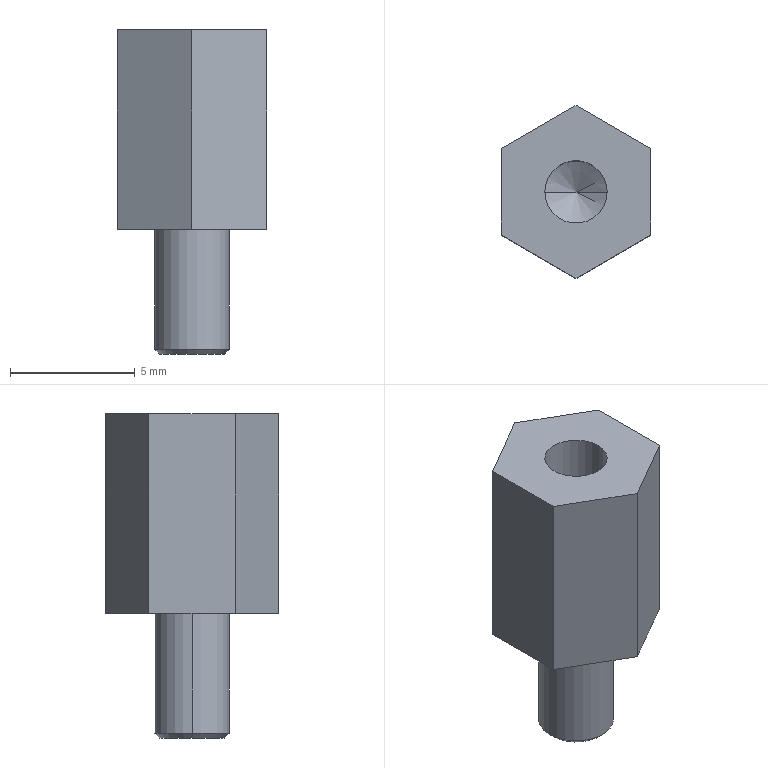Part | STEP file | Brass standoff M3-6x8 | 1 solid | 17 faces | box 6 x 6.928 x 13 mm | volume 251.442 mm3 | plane 9 | cone 4 | cylinder 4 | commonest cylinder face diameters 2.5 x2 3 x2
STEP:
#1=CARTESIAN_POINT('',(0.,0.,0.));
#2=DIRECTION('',(0.,0.,1.));
#3=DIRECTION('',(1.,0.,0.));
#4=AXIS2_PLACEMENT_3D('',#1,#2,#3);
#5=CARTESIAN_POINT('',(-1.3,0.,0.));
#6=VERTEX_POINT('',#5);
#7=CARTESIAN_POINT('',(1.3,0.,0.));
#8=VERTEX_POINT('',#7);
#9=CARTESIAN_POINT('',(0.,0.,0.));
#10=DIRECTION('',(0.,0.,-1.));
#11=DIRECTION('',(1.,0.,0.));
#12=AXIS2_PLACEMENT_3D('',#9,#10,#11);
#13=CIRCLE('',#12,1.3);
#14=CARTESIAN_POINT('',(0.,0.,0.2));
#15=DIRECTION('',(0.,0.,1.));
#16=DIRECTION('',(1.,0.,0.));
#17=AXIS2_PLACEMENT_3D('',#14,#15,#16);
#18=CONICAL_SURFACE('',#17,1.5,0.7854);
#19=CARTESIAN_POINT('',(6.283,-0.2));
#20=DIRECTION('',(-1.,0.));
#21=VECTOR('',#20,1.);
#22=LINE('',#19,#21);
#23=(GEOMETRIC_REPRESENTATION_CONTEXT(2)PARAMETRIC_REPRESENTATION_CONTEXT()REPRESENTATION_CONTEXT('',''));
#24=DEFINITIONAL_REPRESENTATION('',(#22),#23);
#25=PCURVE('',#18,#24);
#26=CARTESIAN_POINT('',(0.,0.,0.));
#27=DIRECTION('',(0.,0.,1.));
#28=DIRECTION('',(1.,0.,0.));
#29=AXIS2_PLACEMENT_3D('',#26,#27,#28);
#30=PLANE('',#29);
#31=CARTESIAN_POINT('',(1.3,0.));
#32=CARTESIAN_POINT('',(1.3,-2.252));
#33=CARTESIAN_POINT('',(-0.65,-1.126));
#34=CARTESIAN_POINT('',(-2.6,0.));
#35=CARTESIAN_POINT('',(-0.65,1.126));
#36=CARTESIAN_POINT('',(1.3,2.252));
#37=CARTESIAN_POINT('',(1.3,0.));
#38=(BOUNDED_CURVE()B_SPLINE_CURVE(2,(#31,#32,#33,#34,#35,#36,#37),.UNSPECIFIED.,.T.,.F.)B_SPLINE_CURVE_WITH_KNOTS((1,2,2,2,2,1),(-2.094,0.,2.094,4.189,6.283,8.378),.UNSPECIFIED.)CURVE()GEOMETRIC_REPRESENTATION_ITEM()RATIONAL_B_SPLINE_CURVE((1.,0.5,1.,0.5,1.,0.5,1.))REPRESENTATION_ITEM(''));
#39=(GEOMETRIC_REPRESENTATION_CONTEXT(2)PARAMETRIC_REPRESENTATION_CONTEXT()REPRESENTATION_CONTEXT('',''));
#40=DEFINITIONAL_REPRESENTATION('',(#38),#39);
#41=PCURVE('',#30,#40);
#42=SURFACE_CURVE('',#13,(#25,#41),.PCURVE_S1.);
#43=EDGE_CURVE('',#6,#8,#42,.T.);
#44=ORIENTED_EDGE('',*,*,#43,.F.);
#45=CARTESIAN_POINT('',(-1.5,0.,0.2));
#46=VERTEX_POINT('',#45);
#47=CARTESIAN_POINT('',(-1.5,0.,0.2));
#48=DIRECTION('',(-0.7071,0.,0.7071));
#49=VECTOR('',#48,1.);
#50=LINE('',#47,#49);
#51=CARTESIAN_POINT('',(3.142,0.));
#52=DIRECTION('',(0.,1.));
#53=VECTOR('',#52,1.);
#54=LINE('',#51,#53);
#55=(GEOMETRIC_REPRESENTATION_CONTEXT(2)PARAMETRIC_REPRESENTATION_CONTEXT()REPRESENTATION_CONTEXT('',''));
#56=DEFINITIONAL_REPRESENTATION('',(#54),#55);
#57=PCURVE('',#18,#56);
#58=CARTESIAN_POINT('',(0.,0.,0.2));
#59=DIRECTION('',(0.,0.,1.));
#60=DIRECTION('',(1.,0.,0.));
#61=AXIS2_PLACEMENT_3D('',#58,#59,#60);
#62=CONICAL_SURFACE('',#61,1.5,0.7854);
#63=CARTESIAN_POINT('',(3.142,0.));
#64=DIRECTION('',(0.,1.));
#65=VECTOR('',#64,1.);
#66=LINE('',#63,#65);
#67=(GEOMETRIC_REPRESENTATION_CONTEXT(2)PARAMETRIC_REPRESENTATION_CONTEXT()REPRESENTATION_CONTEXT('',''));
#68=DEFINITIONAL_REPRESENTATION('',(#66),#67);
#69=PCURVE('',#62,#68);
#70=SURFACE_CURVE('',#50,(#57,#69),.PCURVE_S1.);
#71=EDGE_CURVE('',#6,#46,#70,.T.);
#72=ORIENTED_EDGE('',*,*,#71,.T.);
#73=CARTESIAN_POINT('',(1.5,0.,0.2));
#74=VERTEX_POINT('',#73);
#75=CARTESIAN_POINT('',(0.,0.,0.2));
#76=DIRECTION('',(0.,0.,1.));
#77=DIRECTION('',(1.,0.,0.));
#78=AXIS2_PLACEMENT_3D('',#75,#76,#77);
#79=CIRCLE('',#78,1.5);
#80=CARTESIAN_POINT('',(0.,0.));
#81=DIRECTION('',(1.,0.));
#82=VECTOR('',#81,1.);
#83=LINE('',#80,#82);
#84=(GEOMETRIC_REPRESENTATION_CONTEXT(2)PARAMETRIC_REPRESENTATION_CONTEXT()REPRESENTATION_CONTEXT('',''));
#85=DEFINITIONAL_REPRESENTATION('',(#83),#84);
#86=PCURVE('',#18,#85);
#87=CARTESIAN_POINT('',(0.,0.,5.));
#88=DIRECTION('',(0.,0.,-1.));
#89=DIRECTION('',(-1.,0.,0.));
#90=AXIS2_PLACEMENT_3D('',#87,#88,#89);
#91=CYLINDRICAL_SURFACE('',#90,1.5);
#92=CARTESIAN_POINT('',(3.142,4.8));
#93=DIRECTION('',(-1.,0.));
#94=VECTOR('',#93,1.);
#95=LINE('',#92,#94);
#96=(GEOMETRIC_REPRESENTATION_CONTEXT(2)PARAMETRIC_REPRESENTATION_CONTEXT()REPRESENTATION_CONTEXT('',''));
#97=DEFINITIONAL_REPRESENTATION('',(#95),#96);
#98=PCURVE('',#91,#97);
#99=SURFACE_CURVE('',#79,(#86,#98),.PCURVE_S1.);
#100=EDGE_CURVE('',#74,#46,#99,.T.);
#101=ORIENTED_EDGE('',*,*,#100,.F.);
#102=CARTESIAN_POINT('',(1.5,0.,0.2));
#103=DIRECTION('',(0.7071,0.,0.7071));
#104=VECTOR('',#103,1.);
#105=LINE('',#102,#104);
#106=CARTESIAN_POINT('',(0.,0.));
#107=DIRECTION('',(0.,1.));
#108=VECTOR('',#107,1.);
#109=LINE('',#106,#108);
#110=(GEOMETRIC_REPRESENTATION_CONTEXT(2)PARAMETRIC_REPRESENTATION_CONTEXT()REPRESENTATION_CONTEXT('',''));
#111=DEFINITIONAL_REPRESENTATION('',(#109),#110);
#112=PCURVE('',#18,#111);
#113=CARTESIAN_POINT('',(6.283,0.));
#114=DIRECTION('',(0.,1.));
#115=VECTOR('',#114,1.);
#116=LINE('',#113,#115);
#117=(GEOMETRIC_REPRESENTATION_CONTEXT(2)PARAMETRIC_REPRESENTATION_CONTEXT()REPRESENTATION_CONTEXT('',''));
#118=DEFINITIONAL_REPRESENTATION('',(#116),#117);
#119=PCURVE('',#62,#118);
#120=SURFACE_CURVE('',#105,(#112,#119),.PCURVE_S1.);
#121=EDGE_CURVE('',#8,#74,#120,.T.);
#122=ORIENTED_EDGE('',*,*,#121,.F.);
#123=EDGE_LOOP('',(#44,#72,#101,#122));
#124=FACE_BOUND('',#123,.T.);
#125=ADVANCED_FACE('',(#124),#18,.T.);
#126=CARTESIAN_POINT('',(1.25,0.,6.5));
#127=VERTEX_POINT('',#126);
#128=CARTESIAN_POINT('',(1.25,0.,13.));
#129=VERTEX_POINT('',#128);
#130=CARTESIAN_POINT('',(1.25,0.,13.));
#131=DIRECTION('',(0.,0.,1.));
#132=VECTOR('',#131,1.);
#133=LINE('',#130,#132);
#134=CARTESIAN_POINT('',(0.,0.,13.));
#135=DIRECTION('',(0.,0.,1.));
#136=DIRECTION('',(1.,0.,0.));
#137=AXIS2_PLACEMENT_3D('',#134,#135,#136);
#138=CYLINDRICAL_SURFACE('',#137,1.25);
#139=CARTESIAN_POINT('',(6.283,0.));
#140=DIRECTION('',(0.,1.));
#141=VECTOR('',#140,1.);
#142=LINE('',#139,#141);
#143=(GEOMETRIC_REPRESENTATION_CONTEXT(2)PARAMETRIC_REPRESENTATION_CONTEXT()REPRESENTATION_CONTEXT('',''));
#144=DEFINITIONAL_REPRESENTATION('',(#142),#143);
#145=PCURVE('',#138,#144);
#146=CARTESIAN_POINT('',(0.,0.,13.));
#147=DIRECTION('',(0.,0.,1.));
#148=DIRECTION('',(1.,0.,0.));
#149=AXIS2_PLACEMENT_3D('',#146,#147,#148);
#150=CYLINDRICAL_SURFACE('',#149,1.25);
#151=CARTESIAN_POINT('',(0.,0.));
#152=DIRECTION('',(0.,1.));
#153=VECTOR('',#152,1.);
#154=LINE('',#151,#153);
#155=(GEOMETRIC_REPRESENTATION_CONTEXT(2)PARAMETRIC_REPRESENTATION_CONTEXT()REPRESENTATION_CONTEXT('',''));
#156=DEFINITIONAL_REPRESENTATION('',(#154),#155);
#157=PCURVE('',#150,#156);
#158=SURFACE_CURVE('',#133,(#145,#157),.PCURVE_S1.);
#159=EDGE_CURVE('',#127,#129,#158,.T.);
#160=ORIENTED_EDGE('',*,*,#159,.T.);
#161=CARTESIAN_POINT('',(-1.25,0.,13.));
#162=VERTEX_POINT('',#161);
#163=CARTESIAN_POINT('',(0.,0.,13.));
#164=DIRECTION('',(0.,0.,1.));
#165=DIRECTION('',(1.,0.,0.));
#166=AXIS2_PLACEMENT_3D('',#163,#164,#165);
#167=CIRCLE('',#166,1.25);
#168=CARTESIAN_POINT('',(0.,0.));
#169=DIRECTION('',(1.,0.));
#170=VECTOR('',#169,1.);
#171=LINE('',#168,#170);
#172=(GEOMETRIC_REPRESENTATION_CONTEXT(2)PARAMETRIC_REPRESENTATION_CONTEXT()REPRESENTATION_CONTEXT('',''));
#173=DEFINITIONAL_REPRESENTATION('',(#171),#172);
#174=PCURVE('',#138,#173);
#175=CARTESIAN_POINT('',(3.,-1.732,13.));
#176=DIRECTION('',(0.,0.,1.));
#177=DIRECTION('',(1.,0.,0.));
#178=AXIS2_PLACEMENT_3D('',#175,#176,#177);
#179=PLANE('',#178);
#180=CARTESIAN_POINT('',(-3.,1.732));
#181=DIRECTION('',(1.,0.));
#182=AXIS2_PLACEMENT_2D('',#180,#181);
#183=CIRCLE('',#182,1.25);
#184=(GEOMETRIC_REPRESENTATION_CONTEXT(2)PARAMETRIC_REPRESENTATION_CONTEXT()REPRESENTATION_CONTEXT('',''));
#185=DEFINITIONAL_REPRESENTATION('',(#183),#184);
#186=PCURVE('',#179,#185);
#187=SURFACE_CURVE('',#167,(#174,#186),.PCURVE_S1.);
#188=EDGE_CURVE('',#162,#129,#187,.T.);
#189=ORIENTED_EDGE('',*,*,#188,.F.);
#190=CARTESIAN_POINT('',(-1.25,0.,6.5));
#191=VERTEX_POINT('',#190);
#192=CARTESIAN_POINT('',(-1.25,0.,13.));
#193=DIRECTION('',(0.,0.,1.));
#194=VECTOR('',#193,1.);
#195=LINE('',#192,#194);
#196=CARTESIAN_POINT('',(3.142,0.));
#197=DIRECTION('',(0.,1.));
#198=VECTOR('',#197,1.);
#199=LINE('',#196,#198);
#200=(GEOMETRIC_REPRESENTATION_CONTEXT(2)PARAMETRIC_REPRESENTATION_CONTEXT()REPRESENTATION_CONTEXT('',''));
#201=DEFINITIONAL_REPRESENTATION('',(#199),#200);
#202=PCURVE('',#138,#201);
#203=CARTESIAN_POINT('',(3.142,0.));
#204=DIRECTION('',(0.,1.));
#205=VECTOR('',#204,1.);
#206=LINE('',#203,#205);
#207=(GEOMETRIC_REPRESENTATION_CONTEXT(2)PARAMETRIC_REPRESENTATION_CONTEXT()REPRESENTATION_CONTEXT('',''));
#208=DEFINITIONAL_REPRESENTATION('',(#206),#207);
#209=PCURVE('',#150,#208);
#210=SURFACE_CURVE('',#195,(#202,#209),.PCURVE_S1.);
#211=EDGE_CURVE('',#191,#162,#210,.T.);
#212=ORIENTED_EDGE('',*,*,#211,.F.);
#213=CARTESIAN_POINT('',(0.,0.,6.5));
#214=DIRECTION('',(0.,0.,1.));
#215=DIRECTION('',(1.,0.,0.));
#216=AXIS2_PLACEMENT_3D('',#213,#214,#215);
#217=CIRCLE('',#216,1.25);
#218=CARTESIAN_POINT('',(0.,-6.5));
#219=DIRECTION('',(1.,0.));
#220=VECTOR('',#219,1.);
#221=LINE('',#218,#220);
#222=(GEOMETRIC_REPRESENTATION_CONTEXT(2)PARAMETRIC_REPRESENTATION_CONTEXT()REPRESENTATION_CONTEXT('',''));
#223=DEFINITIONAL_REPRESENTATION('',(#221),#222);
#224=PCURVE('',#138,#223);
#225=CARTESIAN_POINT('',(0.,0.,6.5));
#226=DIRECTION('',(0.,0.,1.));
#227=DIRECTION('',(1.,0.,0.));
#228=AXIS2_PLACEMENT_3D('',#225,#226,#227);
#229=CONICAL_SURFACE('',#228,1.25,1.03);
#230=CARTESIAN_POINT('',(0.,0.));
#231=DIRECTION('',(1.,0.));
#232=VECTOR('',#231,1.);
#233=LINE('',#230,#232);
#234=(GEOMETRIC_REPRESENTATION_CONTEXT(2)PARAMETRIC_REPRESENTATION_CONTEXT()REPRESENTATION_CONTEXT('',''));
#235=DEFINITIONAL_REPRESENTATION('',(#233),#234);
#236=PCURVE('',#229,#235);
#237=SURFACE_CURVE('',#217,(#224,#236),.PCURVE_S1.);
#238=EDGE_CURVE('',#191,#127,#237,.T.);
#239=ORIENTED_EDGE('',*,*,#238,.T.);
#240=EDGE_LOOP('',(#160,#189,#212,#239));
#241=FACE_BOUND('',#240,.F.);
#242=ADVANCED_FACE('',(#241),#138,.F.);
#243=ORIENTED_EDGE('',*,*,#238,.F.);
#244=CARTESIAN_POINT('',(0.,0.,5.749));
#245=VERTEX_POINT('',#244);
#246=CARTESIAN_POINT('',(-1.25,0.,6.5));
#247=DIRECTION('',(-0.8572,0.,0.515));
#248=VECTOR('',#247,1.);
#249=LINE('',#246,#248);
#250=CARTESIAN_POINT('',(3.142,0.));
#251=DIRECTION('',(0.,1.));
#252=VECTOR('',#251,1.);
#253=LINE('',#250,#252);
#254=(GEOMETRIC_REPRESENTATION_CONTEXT(2)PARAMETRIC_REPRESENTATION_CONTEXT()REPRESENTATION_CONTEXT('',''));
#255=DEFINITIONAL_REPRESENTATION('',(#253),#254);
#256=PCURVE('',#229,#255);
#257=CARTESIAN_POINT('',(0.,0.,6.5));
#258=DIRECTION('',(0.,0.,1.));
#259=DIRECTION('',(1.,0.,0.));
#260=AXIS2_PLACEMENT_3D('',#257,#258,#259);
#261=CONICAL_SURFACE('',#260,1.25,1.03);
#262=CARTESIAN_POINT('',(3.142,0.));
#263=DIRECTION('',(0.,1.));
#264=VECTOR('',#263,1.);
#265=LINE('',#262,#264);
#266=(GEOMETRIC_REPRESENTATION_CONTEXT(2)PARAMETRIC_REPRESENTATION_CONTEXT()REPRESENTATION_CONTEXT('',''));
#267=DEFINITIONAL_REPRESENTATION('',(#265),#266);
#268=PCURVE('',#261,#267);
#269=SURFACE_CURVE('',#249,(#256,#268),.PCURVE_S1.);
#270=EDGE_CURVE('',#245,#191,#269,.T.);
#271=ORIENTED_EDGE('',*,*,#270,.F.);
#272=CARTESIAN_POINT('',(1.25,0.,6.5));
#273=DIRECTION('',(0.8572,0.,0.515));
#274=VECTOR('',#273,1.);
#275=LINE('',#272,#274);
#276=CARTESIAN_POINT('',(6.283,0.));
#277=DIRECTION('',(0.,1.));
#278=VECTOR('',#277,1.);
#279=LINE('',#276,#278);
#280=(GEOMETRIC_REPRESENTATION_CONTEXT(2)PARAMETRIC_REPRESENTATION_CONTEXT()REPRESENTATION_CONTEXT('',''));
#281=DEFINITIONAL_REPRESENTATION('',(#279),#280);
#282=PCURVE('',#229,#281);
#283=CARTESIAN_POINT('',(0.,0.));
#284=DIRECTION('',(0.,1.));
#285=VECTOR('',#284,1.);
#286=LINE('',#283,#285);
#287=(GEOMETRIC_REPRESENTATION_CONTEXT(2)PARAMETRIC_REPRESENTATION_CONTEXT()REPRESENTATION_CONTEXT('',''));
#288=DEFINITIONAL_REPRESENTATION('',(#286),#287);
#289=PCURVE('',#261,#288);
#290=SURFACE_CURVE('',#275,(#282,#289),.PCURVE_S1.);
#291=EDGE_CURVE('',#245,#127,#290,.T.);
#292=ORIENTED_EDGE('',*,*,#291,.T.);
#293=EDGE_LOOP('',(#243,#271,#292));
#294=FACE_BOUND('',#293,.F.);
#295=ADVANCED_FACE('',(#294),#229,.F.);
#296=CARTESIAN_POINT('',(1.5,0.,5.));
#297=VERTEX_POINT('',#296);
#298=CARTESIAN_POINT('',(-1.5,0.,5.));
#299=VERTEX_POINT('',#298);
#300=CARTESIAN_POINT('',(0.,0.,5.));
#301=DIRECTION('',(0.,0.,1.));
#302=DIRECTION('',(1.,0.,0.));
#303=AXIS2_PLACEMENT_3D('',#300,#301,#302);
#304=CIRCLE('',#303,1.5);
#305=CARTESIAN_POINT('',(3.142,0.));
#306=DIRECTION('',(-1.,0.));
#307=VECTOR('',#306,1.);
#308=LINE('',#305,#307);
#309=(GEOMETRIC_REPRESENTATION_CONTEXT(2)PARAMETRIC_REPRESENTATION_CONTEXT()REPRESENTATION_CONTEXT('',''));
#310=DEFINITIONAL_REPRESENTATION('',(#308),#309);
#311=PCURVE('',#91,#310);
#312=CARTESIAN_POINT('',(3.,-1.732,5.));
#313=DIRECTION('',(0.,0.,1.));
#314=DIRECTION('',(1.,0.,0.));
#315=AXIS2_PLACEMENT_3D('',#312,#313,#314);
#316=PLANE('',#315);
#317=CARTESIAN_POINT('',(-3.,1.732));
#318=DIRECTION('',(1.,0.));
#319=AXIS2_PLACEMENT_2D('',#317,#318);
#320=CIRCLE('',#319,1.5);
#321=(GEOMETRIC_REPRESENTATION_CONTEXT(2)PARAMETRIC_REPRESENTATION_CONTEXT()REPRESENTATION_CONTEXT('',''));
#322=DEFINITIONAL_REPRESENTATION('',(#320),#321);
#323=PCURVE('',#316,#322);
#324=SURFACE_CURVE('',#304,(#311,#323),.PCURVE_S1.);
#325=EDGE_CURVE('',#297,#299,#324,.T.);
#326=ORIENTED_EDGE('',*,*,#325,.F.);
#327=CARTESIAN_POINT('',(1.5,0.,5.));
#328=DIRECTION('',(0.,0.,-1.));
#329=VECTOR('',#328,1.);
#330=LINE('',#327,#329);
#331=CARTESIAN_POINT('',(3.142,0.));
#332=DIRECTION('',(0.,1.));
#333=VECTOR('',#332,1.);
#334=LINE('',#331,#333);
#335=(GEOMETRIC_REPRESENTATION_CONTEXT(2)PARAMETRIC_REPRESENTATION_CONTEXT()REPRESENTATION_CONTEXT('',''));
#336=DEFINITIONAL_REPRESENTATION('',(#334),#335);
#337=PCURVE('',#91,#336);
#338=CARTESIAN_POINT('',(0.,0.,5.));
#339=DIRECTION('',(0.,0.,-1.));
#340=DIRECTION('',(-1.,0.,0.));
#341=AXIS2_PLACEMENT_3D('',#338,#339,#340);
#342=CYLINDRICAL_SURFACE('',#341,1.5);
#343=CARTESIAN_POINT('',(3.142,0.));
#344=DIRECTION('',(0.,1.));
#345=VECTOR('',#344,1.);
#346=LINE('',#343,#345);
#347=(GEOMETRIC_REPRESENTATION_CONTEXT(2)PARAMETRIC_REPRESENTATION_CONTEXT()REPRESENTATION_CONTEXT('',''));
#348=DEFINITIONAL_REPRESENTATION('',(#346),#347);
#349=PCURVE('',#342,#348);
#350=SURFACE_CURVE('',#330,(#337,#349),.PCURVE_S1.);
#351=EDGE_CURVE('',#297,#74,#350,.T.);
#352=ORIENTED_EDGE('',*,*,#351,.T.);
#353=ORIENTED_EDGE('',*,*,#100,.T.);
#354=CARTESIAN_POINT('',(-1.5,0.,5.));
#355=DIRECTION('',(0.,0.,-1.));
#356=VECTOR('',#355,1.);
#357=LINE('',#354,#356);
#358=CARTESIAN_POINT('',(0.,0.));
#359=DIRECTION('',(0.,1.));
#360=VECTOR('',#359,1.);
#361=LINE('',#358,#360);
#362=(GEOMETRIC_REPRESENTATION_CONTEXT(2)PARAMETRIC_REPRESENTATION_CONTEXT()REPRESENTATION_CONTEXT('',''));
#363=DEFINITIONAL_REPRESENTATION('',(#361),#362);
#364=PCURVE('',#91,#363);
#365=CARTESIAN_POINT('',(6.283,0.));
#366=DIRECTION('',(0.,1.));
#367=VECTOR('',#366,1.);
#368=LINE('',#365,#367);
#369=(GEOMETRIC_REPRESENTATION_CONTEXT(2)PARAMETRIC_REPRESENTATION_CONTEXT()REPRESENTATION_CONTEXT('',''));
#370=DEFINITIONAL_REPRESENTATION('',(#368),#369);
#371=PCURVE('',#342,#370);
#372=SURFACE_CURVE('',#357,(#364,#371),.PCURVE_S1.);
#373=EDGE_CURVE('',#299,#46,#372,.T.);
#374=ORIENTED_EDGE('',*,*,#373,.F.);
#375=EDGE_LOOP('',(#326,#352,#353,#374));
#376=FACE_BOUND('',#375,.T.);
#377=ADVANCED_FACE('',(#376),#91,.T.);
#378=ORIENTED_EDGE('',*,*,#351,.F.);
#379=CARTESIAN_POINT('',(0.,0.,5.));
#380=DIRECTION('',(0.,0.,1.));
#381=DIRECTION('',(1.,0.,0.));
#382=AXIS2_PLACEMENT_3D('',#379,#380,#381);
#383=CIRCLE('',#382,1.5);
#384=CARTESIAN_POINT('',(9.425,0.));
#385=DIRECTION('',(-1.,0.));
#386=VECTOR('',#385,1.);
#387=LINE('',#384,#386);
#388=(GEOMETRIC_REPRESENTATION_CONTEXT(2)PARAMETRIC_REPRESENTATION_CONTEXT()REPRESENTATION_CONTEXT('',''));
#389=DEFINITIONAL_REPRESENTATION('',(#387),#388);
#390=PCURVE('',#342,#389);
#391=CARTESIAN_POINT('',(-3.,1.732));
#392=DIRECTION('',(1.,0.));
#393=AXIS2_PLACEMENT_2D('',#391,#392);
#394=CIRCLE('',#393,1.5);
#395=(GEOMETRIC_REPRESENTATION_CONTEXT(2)PARAMETRIC_REPRESENTATION_CONTEXT()REPRESENTATION_CONTEXT('',''));
#396=DEFINITIONAL_REPRESENTATION('',(#394),#395);
#397=PCURVE('',#316,#396);
#398=SURFACE_CURVE('',#383,(#390,#397),.PCURVE_S1.);
#399=EDGE_CURVE('',#299,#297,#398,.T.);
#400=ORIENTED_EDGE('',*,*,#399,.F.);
#401=ORIENTED_EDGE('',*,*,#373,.T.);
#402=CARTESIAN_POINT('',(0.,0.,0.2));
#403=DIRECTION('',(0.,0.,1.));
#404=DIRECTION('',(1.,0.,0.));
#405=AXIS2_PLACEMENT_3D('',#402,#403,#404);
#406=CIRCLE('',#405,1.5);
#407=CARTESIAN_POINT('',(9.425,4.8));
#408=DIRECTION('',(-1.,0.));
#409=VECTOR('',#408,1.);
#410=LINE('',#407,#409);
#411=(GEOMETRIC_REPRESENTATION_CONTEXT(2)PARAMETRIC_REPRESENTATION_CONTEXT()REPRESENTATION_CONTEXT('',''));
#412=DEFINITIONAL_REPRESENTATION('',(#410),#411);
#413=PCURVE('',#342,#412);
#414=CARTESIAN_POINT('',(0.,0.));
#415=DIRECTION('',(1.,0.));
#416=VECTOR('',#415,1.);
#417=LINE('',#414,#416);
#418=(GEOMETRIC_REPRESENTATION_CONTEXT(2)PARAMETRIC_REPRESENTATION_CONTEXT()REPRESENTATION_CONTEXT('',''));
#419=DEFINITIONAL_REPRESENTATION('',(#417),#418);
#420=PCURVE('',#62,#419);
#421=SURFACE_CURVE('',#406,(#413,#420),.PCURVE_S1.);
#422=EDGE_CURVE('',#46,#74,#421,.T.);
#423=ORIENTED_EDGE('',*,*,#422,.T.);
#424=EDGE_LOOP('',(#378,#400,#401,#423));
#425=FACE_BOUND('',#424,.T.);
#426=ADVANCED_FACE('',(#425),#342,.T.);
#427=CARTESIAN_POINT('',(0.,0.,0.));
#428=DIRECTION('',(0.,0.,-1.));
#429=DIRECTION('',(1.,0.,0.));
#430=AXIS2_PLACEMENT_3D('',#427,#428,#429);
#431=CIRCLE('',#430,1.3);
#432=CARTESIAN_POINT('',(1.3,0.));
#433=CARTESIAN_POINT('',(1.3,-2.252));
#434=CARTESIAN_POINT('',(-0.65,-1.126));
#435=CARTESIAN_POINT('',(-2.6,0.));
#436=CARTESIAN_POINT('',(-0.65,1.126));
#437=CARTESIAN_POINT('',(1.3,2.252));
#438=CARTESIAN_POINT('',(1.3,0.));
#439=(BOUNDED_CURVE()B_SPLINE_CURVE(2,(#432,#433,#434,#435,#436,#437,#438),.UNSPECIFIED.,.T.,.F.)B_SPLINE_CURVE_WITH_KNOTS((1,2,2,2,2,1),(-2.094,0.,2.094,4.189,6.283,8.378),.UNSPECIFIED.)CURVE()GEOMETRIC_REPRESENTATION_ITEM()RATIONAL_B_SPLINE_CURVE((1.,0.5,1.,0.5,1.,0.5,1.))REPRESENTATION_ITEM(''));
#440=(GEOMETRIC_REPRESENTATION_CONTEXT(2)PARAMETRIC_REPRESENTATION_CONTEXT()REPRESENTATION_CONTEXT('',''));
#441=DEFINITIONAL_REPRESENTATION('',(#439),#440);
#442=PCURVE('',#30,#441);
#443=CARTESIAN_POINT('',(6.283,-0.2));
#444=DIRECTION('',(-1.,0.));
#445=VECTOR('',#444,1.);
#446=LINE('',#443,#445);
#447=(GEOMETRIC_REPRESENTATION_CONTEXT(2)PARAMETRIC_REPRESENTATION_CONTEXT()REPRESENTATION_CONTEXT('',''));
#448=DEFINITIONAL_REPRESENTATION('',(#446),#447);
#449=PCURVE('',#62,#448);
#450=SURFACE_CURVE('',#431,(#442,#449),.PCURVE_S1.);
#451=EDGE_CURVE('',#8,#6,#450,.T.);
#452=ORIENTED_EDGE('',*,*,#451,.T.);
#453=ORIENTED_EDGE('',*,*,#43,.T.);
#454=EDGE_LOOP('',(#452,#453));
#455=FACE_BOUND('',#454,.T.);
#456=ADVANCED_FACE('',(#455),#30,.F.);
#457=CARTESIAN_POINT('',(0.,-3.464,5.));
#458=VERTEX_POINT('',#457);
#459=CARTESIAN_POINT('',(3.,-1.732,5.));
#460=VERTEX_POINT('',#459);
#461=CARTESIAN_POINT('',(0.,-3.464,5.));
#462=DIRECTION('',(0.866,0.5,0.));
#463=VECTOR('',#462,1.);
#464=LINE('',#461,#463);
#465=CARTESIAN_POINT('',(-3.,-1.732));
#466=DIRECTION('',(0.866,0.5));
#467=VECTOR('',#466,1.);
#468=LINE('',#465,#467);
#469=(GEOMETRIC_REPRESENTATION_CONTEXT(2)PARAMETRIC_REPRESENTATION_CONTEXT()REPRESENTATION_CONTEXT('',''));
#470=DEFINITIONAL_REPRESENTATION('',(#468),#469);
#471=PCURVE('',#316,#470);
#472=CARTESIAN_POINT('',(0.,-3.464,13.));
#473=DIRECTION('',(-0.5,0.866,0.));
#474=DIRECTION('',(-0.866,-0.5,0.));
#475=AXIS2_PLACEMENT_3D('',#472,#473,#474);
#476=PLANE('',#475);
#477=CARTESIAN_POINT('',(0.,-8.));
#478=DIRECTION('',(-1.,0.));
#479=VECTOR('',#478,1.);
#480=LINE('',#477,#479);
#481=(GEOMETRIC_REPRESENTATION_CONTEXT(2)PARAMETRIC_REPRESENTATION_CONTEXT()REPRESENTATION_CONTEXT('',''));
#482=DEFINITIONAL_REPRESENTATION('',(#480),#481);
#483=PCURVE('',#476,#482);
#484=SURFACE_CURVE('',#464,(#471,#483),.PCURVE_S1.);
#485=EDGE_CURVE('',#458,#460,#484,.T.);
#486=ORIENTED_EDGE('',*,*,#485,.F.);
#487=CARTESIAN_POINT('',(-3.,-1.732,5.));
#488=VERTEX_POINT('',#487);
#489=CARTESIAN_POINT('',(-3.,-1.732,5.));
#490=DIRECTION('',(0.866,-0.5,0.));
#491=VECTOR('',#490,1.);
#492=LINE('',#489,#491);
#493=CARTESIAN_POINT('',(-6.,0.));
#494=DIRECTION('',(0.866,-0.5));
#495=VECTOR('',#494,1.);
#496=LINE('',#493,#495);
#497=(GEOMETRIC_REPRESENTATION_CONTEXT(2)PARAMETRIC_REPRESENTATION_CONTEXT()REPRESENTATION_CONTEXT('',''));
#498=DEFINITIONAL_REPRESENTATION('',(#496),#497);
#499=PCURVE('',#316,#498);
#500=CARTESIAN_POINT('',(-3.,-1.732,13.));
#501=DIRECTION('',(0.5,0.866,0.));
#502=DIRECTION('',(-0.866,0.5,0.));
#503=AXIS2_PLACEMENT_3D('',#500,#501,#502);
#504=PLANE('',#503);
#505=CARTESIAN_POINT('',(0.,-8.));
#506=DIRECTION('',(-1.,0.));
#507=VECTOR('',#506,1.);
#508=LINE('',#505,#507);
#509=(GEOMETRIC_REPRESENTATION_CONTEXT(2)PARAMETRIC_REPRESENTATION_CONTEXT()REPRESENTATION_CONTEXT('',''));
#510=DEFINITIONAL_REPRESENTATION('',(#508),#509);
#511=PCURVE('',#504,#510);
#512=SURFACE_CURVE('',#492,(#499,#511),.PCURVE_S1.);
#513=EDGE_CURVE('',#488,#458,#512,.T.);
#514=ORIENTED_EDGE('',*,*,#513,.F.);
#515=CARTESIAN_POINT('',(-3.,1.732,5.));
#516=VERTEX_POINT('',#515);
#517=CARTESIAN_POINT('',(-3.,1.732,5.));
#518=DIRECTION('',(0.,-1.,0.));
#519=VECTOR('',#518,1.);
#520=LINE('',#517,#519);
#521=CARTESIAN_POINT('',(-6.,3.464));
#522=DIRECTION('',(0.,-1.));
#523=VECTOR('',#522,1.);
#524=LINE('',#521,#523);
#525=(GEOMETRIC_REPRESENTATION_CONTEXT(2)PARAMETRIC_REPRESENTATION_CONTEXT()REPRESENTATION_CONTEXT('',''));
#526=DEFINITIONAL_REPRESENTATION('',(#524),#525);
#527=PCURVE('',#316,#526);
#528=CARTESIAN_POINT('',(-3.,1.732,13.));
#529=DIRECTION('',(1.,0.,0.));
#530=DIRECTION('',(0.,0.,-1.));
#531=AXIS2_PLACEMENT_3D('',#528,#529,#530);
#532=PLANE('',#531);
#533=CARTESIAN_POINT('',(8.,0.));
#534=DIRECTION('',(0.,-1.));
#535=VECTOR('',#534,1.);
#536=LINE('',#533,#535);
#537=(GEOMETRIC_REPRESENTATION_CONTEXT(2)PARAMETRIC_REPRESENTATION_CONTEXT()REPRESENTATION_CONTEXT('',''));
#538=DEFINITIONAL_REPRESENTATION('',(#536),#537);
#539=PCURVE('',#532,#538);
#540=SURFACE_CURVE('',#520,(#527,#539),.PCURVE_S1.);
#541=EDGE_CURVE('',#516,#488,#540,.T.);
#542=ORIENTED_EDGE('',*,*,#541,.F.);
#543=CARTESIAN_POINT('',(0.,3.464,5.));
#544=VERTEX_POINT('',#543);
#545=CARTESIAN_POINT('',(0.,3.464,5.));
#546=DIRECTION('',(-0.866,-0.5,0.));
#547=VECTOR('',#546,1.);
#548=LINE('',#545,#547);
#549=CARTESIAN_POINT('',(-3.,5.196));
#550=DIRECTION('',(-0.866,-0.5));
#551=VECTOR('',#550,1.);
#552=LINE('',#549,#551);
#553=(GEOMETRIC_REPRESENTATION_CONTEXT(2)PARAMETRIC_REPRESENTATION_CONTEXT()REPRESENTATION_CONTEXT('',''));
#554=DEFINITIONAL_REPRESENTATION('',(#552),#553);
#555=PCURVE('',#316,#554);
#556=CARTESIAN_POINT('',(0.,3.464,13.));
#557=DIRECTION('',(0.5,-0.866,0.));
#558=DIRECTION('',(0.866,0.5,0.));
#559=AXIS2_PLACEMENT_3D('',#556,#557,#558);
#560=PLANE('',#559);
#561=CARTESIAN_POINT('',(0.,-8.));
#562=DIRECTION('',(-1.,0.));
#563=VECTOR('',#562,1.);
#564=LINE('',#561,#563);
#565=(GEOMETRIC_REPRESENTATION_CONTEXT(2)PARAMETRIC_REPRESENTATION_CONTEXT()REPRESENTATION_CONTEXT('',''));
#566=DEFINITIONAL_REPRESENTATION('',(#564),#565);
#567=PCURVE('',#560,#566);
#568=SURFACE_CURVE('',#548,(#555,#567),.PCURVE_S1.);
#569=EDGE_CURVE('',#544,#516,#568,.T.);
#570=ORIENTED_EDGE('',*,*,#569,.F.);
#571=CARTESIAN_POINT('',(3.,1.732,5.));
#572=VERTEX_POINT('',#571);
#573=CARTESIAN_POINT('',(3.,1.732,5.));
#574=DIRECTION('',(-0.866,0.5,0.));
#575=VECTOR('',#574,1.);
#576=LINE('',#573,#575);
#577=CARTESIAN_POINT('',(0.,3.464));
#578=DIRECTION('',(-0.866,0.5));
#579=VECTOR('',#578,1.);
#580=LINE('',#577,#579);
#581=(GEOMETRIC_REPRESENTATION_CONTEXT(2)PARAMETRIC_REPRESENTATION_CONTEXT()REPRESENTATION_CONTEXT('',''));
#582=DEFINITIONAL_REPRESENTATION('',(#580),#581);
#583=PCURVE('',#316,#582);
#584=CARTESIAN_POINT('',(3.,1.732,13.));
#585=DIRECTION('',(-0.5,-0.866,0.));
#586=DIRECTION('',(0.866,-0.5,0.));
#587=AXIS2_PLACEMENT_3D('',#584,#585,#586);
#588=PLANE('',#587);
#589=CARTESIAN_POINT('',(0.,-8.));
#590=DIRECTION('',(-1.,0.));
#591=VECTOR('',#590,1.);
#592=LINE('',#589,#591);
#593=(GEOMETRIC_REPRESENTATION_CONTEXT(2)PARAMETRIC_REPRESENTATION_CONTEXT()REPRESENTATION_CONTEXT('',''));
#594=DEFINITIONAL_REPRESENTATION('',(#592),#593);
#595=PCURVE('',#588,#594);
#596=SURFACE_CURVE('',#576,(#583,#595),.PCURVE_S1.);
#597=EDGE_CURVE('',#572,#544,#596,.T.);
#598=ORIENTED_EDGE('',*,*,#597,.F.);
#599=CARTESIAN_POINT('',(3.,-1.732,5.));
#600=DIRECTION('',(0.,1.,0.));
#601=VECTOR('',#600,1.);
#602=LINE('',#599,#601);
#603=CARTESIAN_POINT('',(0.,0.));
#604=DIRECTION('',(0.,1.));
#605=VECTOR('',#604,1.);
#606=LINE('',#603,#605);
#607=(GEOMETRIC_REPRESENTATION_CONTEXT(2)PARAMETRIC_REPRESENTATION_CONTEXT()REPRESENTATION_CONTEXT('',''));
#608=DEFINITIONAL_REPRESENTATION('',(#606),#607);
#609=PCURVE('',#316,#608);
#610=CARTESIAN_POINT('',(3.,-1.732,13.));
#611=DIRECTION('',(-1.,0.,0.));
#612=DIRECTION('',(0.,0.,1.));
#613=AXIS2_PLACEMENT_3D('',#610,#611,#612);
#614=PLANE('',#613);
#615=CARTESIAN_POINT('',(-8.,0.));
#616=DIRECTION('',(0.,1.));
#617=VECTOR('',#616,1.);
#618=LINE('',#615,#617);
#619=(GEOMETRIC_REPRESENTATION_CONTEXT(2)PARAMETRIC_REPRESENTATION_CONTEXT()REPRESENTATION_CONTEXT('',''));
#620=DEFINITIONAL_REPRESENTATION('',(#618),#619);
#621=PCURVE('',#614,#620);
#622=SURFACE_CURVE('',#602,(#609,#621),.PCURVE_S1.);
#623=EDGE_CURVE('',#460,#572,#622,.T.);
#624=ORIENTED_EDGE('',*,*,#623,.F.);
#625=EDGE_LOOP('',(#486,#514,#542,#570,#598,#624));
#626=FACE_BOUND('',#625,.T.);
#627=ORIENTED_EDGE('',*,*,#399,.T.);
#628=ORIENTED_EDGE('',*,*,#325,.T.);
#629=EDGE_LOOP('',(#627,#628));
#630=FACE_BOUND('',#629,.T.);
#631=ADVANCED_FACE('',(#626,#630),#316,.F.);
#632=ORIENTED_EDGE('',*,*,#485,.T.);
#633=CARTESIAN_POINT('',(3.,-1.732,13.));
#634=VERTEX_POINT('',#633);
#635=CARTESIAN_POINT('',(3.,-1.732,13.));
#636=DIRECTION('',(0.,0.,-1.));
#637=VECTOR('',#636,1.);
#638=LINE('',#635,#637);
#639=CARTESIAN_POINT('',(-3.464,0.));
#640=DIRECTION('',(0.,-1.));
#641=VECTOR('',#640,1.);
#642=LINE('',#639,#641);
#643=(GEOMETRIC_REPRESENTATION_CONTEXT(2)PARAMETRIC_REPRESENTATION_CONTEXT()REPRESENTATION_CONTEXT('',''));
#644=DEFINITIONAL_REPRESENTATION('',(#642),#643);
#645=PCURVE('',#476,#644);
#646=CARTESIAN_POINT('',(0.,0.));
#647=DIRECTION('',(-1.,0.));
#648=VECTOR('',#647,1.);
#649=LINE('',#646,#648);
#650=(GEOMETRIC_REPRESENTATION_CONTEXT(2)PARAMETRIC_REPRESENTATION_CONTEXT()REPRESENTATION_CONTEXT('',''));
#651=DEFINITIONAL_REPRESENTATION('',(#649),#650);
#652=PCURVE('',#614,#651);
#653=SURFACE_CURVE('',#638,(#645,#652),.PCURVE_S1.);
#654=EDGE_CURVE('',#634,#460,#653,.T.);
#655=ORIENTED_EDGE('',*,*,#654,.F.);
#656=CARTESIAN_POINT('',(0.,-3.464,13.));
#657=VERTEX_POINT('',#656);
#658=CARTESIAN_POINT('',(0.,-3.464,13.));
#659=DIRECTION('',(0.866,0.5,0.));
#660=VECTOR('',#659,1.);
#661=LINE('',#658,#660);
#662=CARTESIAN_POINT('',(0.,0.));
#663=DIRECTION('',(-1.,0.));
#664=VECTOR('',#663,1.);
#665=LINE('',#662,#664);
#666=(GEOMETRIC_REPRESENTATION_CONTEXT(2)PARAMETRIC_REPRESENTATION_CONTEXT()REPRESENTATION_CONTEXT('',''));
#667=DEFINITIONAL_REPRESENTATION('',(#665),#666);
#668=PCURVE('',#476,#667);
#669=CARTESIAN_POINT('',(-3.,-1.732));
#670=DIRECTION('',(0.866,0.5));
#671=VECTOR('',#670,1.);
#672=LINE('',#669,#671);
#673=(GEOMETRIC_REPRESENTATION_CONTEXT(2)PARAMETRIC_REPRESENTATION_CONTEXT()REPRESENTATION_CONTEXT('',''));
#674=DEFINITIONAL_REPRESENTATION('',(#672),#673);
#675=PCURVE('',#179,#674);
#676=SURFACE_CURVE('',#661,(#668,#675),.PCURVE_S1.);
#677=EDGE_CURVE('',#657,#634,#676,.T.);
#678=ORIENTED_EDGE('',*,*,#677,.F.);
#679=CARTESIAN_POINT('',(0.,-3.464,13.));
#680=DIRECTION('',(0.,0.,-1.));
#681=VECTOR('',#680,1.);
#682=LINE('',#679,#681);
#683=CARTESIAN_POINT('',(0.,0.));
#684=DIRECTION('',(0.,-1.));
#685=VECTOR('',#684,1.);
#686=LINE('',#683,#685);
#687=(GEOMETRIC_REPRESENTATION_CONTEXT(2)PARAMETRIC_REPRESENTATION_CONTEXT()REPRESENTATION_CONTEXT('',''));
#688=DEFINITIONAL_REPRESENTATION('',(#686),#687);
#689=PCURVE('',#476,#688);
#690=CARTESIAN_POINT('',(-3.464,0.));
#691=DIRECTION('',(0.,-1.));
#692=VECTOR('',#691,1.);
#693=LINE('',#690,#692);
#694=(GEOMETRIC_REPRESENTATION_CONTEXT(2)PARAMETRIC_REPRESENTATION_CONTEXT()REPRESENTATION_CONTEXT('',''));
#695=DEFINITIONAL_REPRESENTATION('',(#693),#694);
#696=PCURVE('',#504,#695);
#697=SURFACE_CURVE('',#682,(#689,#696),.PCURVE_S1.);
#698=EDGE_CURVE('',#657,#458,#697,.T.);
#699=ORIENTED_EDGE('',*,*,#698,.T.);
#700=EDGE_LOOP('',(#632,#655,#678,#699));
#701=FACE_BOUND('',#700,.T.);
#702=ADVANCED_FACE('',(#701),#476,.F.);
#703=ORIENTED_EDGE('',*,*,#623,.T.);
#704=CARTESIAN_POINT('',(3.,1.732,13.));
#705=VERTEX_POINT('',#704);
#706=CARTESIAN_POINT('',(3.,1.732,13.));
#707=DIRECTION('',(0.,0.,-1.));
#708=VECTOR('',#707,1.);
#709=LINE('',#706,#708);
#710=CARTESIAN_POINT('',(0.,3.464));
#711=DIRECTION('',(-1.,0.));
#712=VECTOR('',#711,1.);
#713=LINE('',#710,#712);
#714=(GEOMETRIC_REPRESENTATION_CONTEXT(2)PARAMETRIC_REPRESENTATION_CONTEXT()REPRESENTATION_CONTEXT('',''));
#715=DEFINITIONAL_REPRESENTATION('',(#713),#714);
#716=PCURVE('',#614,#715);
#717=CARTESIAN_POINT('',(0.,0.));
#718=DIRECTION('',(0.,-1.));
#719=VECTOR('',#718,1.);
#720=LINE('',#717,#719);
#721=(GEOMETRIC_REPRESENTATION_CONTEXT(2)PARAMETRIC_REPRESENTATION_CONTEXT()REPRESENTATION_CONTEXT('',''));
#722=DEFINITIONAL_REPRESENTATION('',(#720),#721);
#723=PCURVE('',#588,#722);
#724=SURFACE_CURVE('',#709,(#716,#723),.PCURVE_S1.);
#725=EDGE_CURVE('',#705,#572,#724,.T.);
#726=ORIENTED_EDGE('',*,*,#725,.F.);
#727=CARTESIAN_POINT('',(3.,-1.732,13.));
#728=DIRECTION('',(0.,1.,0.));
#729=VECTOR('',#728,1.);
#730=LINE('',#727,#729);
#731=CARTESIAN_POINT('',(0.,0.));
#732=DIRECTION('',(0.,1.));
#733=VECTOR('',#732,1.);
#734=LINE('',#731,#733);
#735=(GEOMETRIC_REPRESENTATION_CONTEXT(2)PARAMETRIC_REPRESENTATION_CONTEXT()REPRESENTATION_CONTEXT('',''));
#736=DEFINITIONAL_REPRESENTATION('',(#734),#735);
#737=PCURVE('',#614,#736);
#738=CARTESIAN_POINT('',(0.,0.));
#739=DIRECTION('',(0.,1.));
#740=VECTOR('',#739,1.);
#741=LINE('',#738,#740);
#742=(GEOMETRIC_REPRESENTATION_CONTEXT(2)PARAMETRIC_REPRESENTATION_CONTEXT()REPRESENTATION_CONTEXT('',''));
#743=DEFINITIONAL_REPRESENTATION('',(#741),#742);
#744=PCURVE('',#179,#743);
#745=SURFACE_CURVE('',#730,(#737,#744),.PCURVE_S1.);
#746=EDGE_CURVE('',#634,#705,#745,.T.);
#747=ORIENTED_EDGE('',*,*,#746,.F.);
#748=ORIENTED_EDGE('',*,*,#654,.T.);
#749=EDGE_LOOP('',(#703,#726,#747,#748));
#750=FACE_BOUND('',#749,.T.);
#751=ADVANCED_FACE('',(#750),#614,.F.);
#752=ORIENTED_EDGE('',*,*,#597,.T.);
#753=CARTESIAN_POINT('',(0.,3.464,13.));
#754=VERTEX_POINT('',#753);
#755=CARTESIAN_POINT('',(0.,3.464,13.));
#756=DIRECTION('',(0.,0.,-1.));
#757=VECTOR('',#756,1.);
#758=LINE('',#755,#757);
#759=CARTESIAN_POINT('',(-3.464,0.));
#760=DIRECTION('',(0.,-1.));
#761=VECTOR('',#760,1.);
#762=LINE('',#759,#761);
#763=(GEOMETRIC_REPRESENTATION_CONTEXT(2)PARAMETRIC_REPRESENTATION_CONTEXT()REPRESENTATION_CONTEXT('',''));
#764=DEFINITIONAL_REPRESENTATION('',(#762),#763);
#765=PCURVE('',#588,#764);
#766=CARTESIAN_POINT('',(0.,0.));
#767=DIRECTION('',(0.,-1.));
#768=VECTOR('',#767,1.);
#769=LINE('',#766,#768);
#770=(GEOMETRIC_REPRESENTATION_CONTEXT(2)PARAMETRIC_REPRESENTATION_CONTEXT()REPRESENTATION_CONTEXT('',''));
#771=DEFINITIONAL_REPRESENTATION('',(#769),#770);
#772=PCURVE('',#560,#771);
#773=SURFACE_CURVE('',#758,(#765,#772),.PCURVE_S1.);
#774=EDGE_CURVE('',#754,#544,#773,.T.);
#775=ORIENTED_EDGE('',*,*,#774,.F.);
#776=CARTESIAN_POINT('',(3.,1.732,13.));
#777=DIRECTION('',(-0.866,0.5,0.));
#778=VECTOR('',#777,1.);
#779=LINE('',#776,#778);
#780=CARTESIAN_POINT('',(0.,0.));
#781=DIRECTION('',(-1.,0.));
#782=VECTOR('',#781,1.);
#783=LINE('',#780,#782);
#784=(GEOMETRIC_REPRESENTATION_CONTEXT(2)PARAMETRIC_REPRESENTATION_CONTEXT()REPRESENTATION_CONTEXT('',''));
#785=DEFINITIONAL_REPRESENTATION('',(#783),#784);
#786=PCURVE('',#588,#785);
#787=CARTESIAN_POINT('',(0.,3.464));
#788=DIRECTION('',(-0.866,0.5));
#789=VECTOR('',#788,1.);
#790=LINE('',#787,#789);
#791=(GEOMETRIC_REPRESENTATION_CONTEXT(2)PARAMETRIC_REPRESENTATION_CONTEXT()REPRESENTATION_CONTEXT('',''));
#792=DEFINITIONAL_REPRESENTATION('',(#790),#791);
#793=PCURVE('',#179,#792);
#794=SURFACE_CURVE('',#779,(#786,#793),.PCURVE_S1.);
#795=EDGE_CURVE('',#705,#754,#794,.T.);
#796=ORIENTED_EDGE('',*,*,#795,.F.);
#797=ORIENTED_EDGE('',*,*,#725,.T.);
#798=EDGE_LOOP('',(#752,#775,#796,#797));
#799=FACE_BOUND('',#798,.T.);
#800=ADVANCED_FACE('',(#799),#588,.F.);
#801=ORIENTED_EDGE('',*,*,#569,.T.);
#802=CARTESIAN_POINT('',(-3.,1.732,13.));
#803=VERTEX_POINT('',#802);
#804=CARTESIAN_POINT('',(-3.,1.732,13.));
#805=DIRECTION('',(0.,0.,-1.));
#806=VECTOR('',#805,1.);
#807=LINE('',#804,#806);
#808=CARTESIAN_POINT('',(-3.464,0.));
#809=DIRECTION('',(0.,-1.));
#810=VECTOR('',#809,1.);
#811=LINE('',#808,#810);
#812=(GEOMETRIC_REPRESENTATION_CONTEXT(2)PARAMETRIC_REPRESENTATION_CONTEXT()REPRESENTATION_CONTEXT('',''));
#813=DEFINITIONAL_REPRESENTATION('',(#811),#812);
#814=PCURVE('',#560,#813);
#815=CARTESIAN_POINT('',(0.,0.));
#816=DIRECTION('',(1.,0.));
#817=VECTOR('',#816,1.);
#818=LINE('',#815,#817);
#819=(GEOMETRIC_REPRESENTATION_CONTEXT(2)PARAMETRIC_REPRESENTATION_CONTEXT()REPRESENTATION_CONTEXT('',''));
#820=DEFINITIONAL_REPRESENTATION('',(#818),#819);
#821=PCURVE('',#532,#820);
#822=SURFACE_CURVE('',#807,(#814,#821),.PCURVE_S1.);
#823=EDGE_CURVE('',#803,#516,#822,.T.);
#824=ORIENTED_EDGE('',*,*,#823,.F.);
#825=CARTESIAN_POINT('',(0.,3.464,13.));
#826=DIRECTION('',(-0.866,-0.5,0.));
#827=VECTOR('',#826,1.);
#828=LINE('',#825,#827);
#829=CARTESIAN_POINT('',(0.,0.));
#830=DIRECTION('',(-1.,0.));
#831=VECTOR('',#830,1.);
#832=LINE('',#829,#831);
#833=(GEOMETRIC_REPRESENTATION_CONTEXT(2)PARAMETRIC_REPRESENTATION_CONTEXT()REPRESENTATION_CONTEXT('',''));
#834=DEFINITIONAL_REPRESENTATION('',(#832),#833);
#835=PCURVE('',#560,#834);
#836=CARTESIAN_POINT('',(-3.,5.196));
#837=DIRECTION('',(-0.866,-0.5));
#838=VECTOR('',#837,1.);
#839=LINE('',#836,#838);
#840=(GEOMETRIC_REPRESENTATION_CONTEXT(2)PARAMETRIC_REPRESENTATION_CONTEXT()REPRESENTATION_CONTEXT('',''));
#841=DEFINITIONAL_REPRESENTATION('',(#839),#840);
#842=PCURVE('',#179,#841);
#843=SURFACE_CURVE('',#828,(#835,#842),.PCURVE_S1.);
#844=EDGE_CURVE('',#754,#803,#843,.T.);
#845=ORIENTED_EDGE('',*,*,#844,.F.);
#846=ORIENTED_EDGE('',*,*,#774,.T.);
#847=EDGE_LOOP('',(#801,#824,#845,#846));
#848=FACE_BOUND('',#847,.T.);
#849=ADVANCED_FACE('',(#848),#560,.F.);
#850=ORIENTED_EDGE('',*,*,#541,.T.);
#851=CARTESIAN_POINT('',(-3.,-1.732,13.));
#852=VERTEX_POINT('',#851);
#853=CARTESIAN_POINT('',(-3.,-1.732,13.));
#854=DIRECTION('',(0.,0.,-1.));
#855=VECTOR('',#854,1.);
#856=LINE('',#853,#855);
#857=CARTESIAN_POINT('',(0.,-3.464));
#858=DIRECTION('',(1.,0.));
#859=VECTOR('',#858,1.);
#860=LINE('',#857,#859);
#861=(GEOMETRIC_REPRESENTATION_CONTEXT(2)PARAMETRIC_REPRESENTATION_CONTEXT()REPRESENTATION_CONTEXT('',''));
#862=DEFINITIONAL_REPRESENTATION('',(#860),#861);
#863=PCURVE('',#532,#862);
#864=CARTESIAN_POINT('',(0.,0.));
#865=DIRECTION('',(0.,-1.));
#866=VECTOR('',#865,1.);
#867=LINE('',#864,#866);
#868=(GEOMETRIC_REPRESENTATION_CONTEXT(2)PARAMETRIC_REPRESENTATION_CONTEXT()REPRESENTATION_CONTEXT('',''));
#869=DEFINITIONAL_REPRESENTATION('',(#867),#868);
#870=PCURVE('',#504,#869);
#871=SURFACE_CURVE('',#856,(#863,#870),.PCURVE_S1.);
#872=EDGE_CURVE('',#852,#488,#871,.T.);
#873=ORIENTED_EDGE('',*,*,#872,.F.);
#874=CARTESIAN_POINT('',(-3.,1.732,13.));
#875=DIRECTION('',(0.,-1.,0.));
#876=VECTOR('',#875,1.);
#877=LINE('',#874,#876);
#878=CARTESIAN_POINT('',(0.,0.));
#879=DIRECTION('',(0.,-1.));
#880=VECTOR('',#879,1.);
#881=LINE('',#878,#880);
#882=(GEOMETRIC_REPRESENTATION_CONTEXT(2)PARAMETRIC_REPRESENTATION_CONTEXT()REPRESENTATION_CONTEXT('',''));
#883=DEFINITIONAL_REPRESENTATION('',(#881),#882);
#884=PCURVE('',#532,#883);
#885=CARTESIAN_POINT('',(-6.,3.464));
#886=DIRECTION('',(0.,-1.));
#887=VECTOR('',#886,1.);
#888=LINE('',#885,#887);
#889=(GEOMETRIC_REPRESENTATION_CONTEXT(2)PARAMETRIC_REPRESENTATION_CONTEXT()REPRESENTATION_CONTEXT('',''));
#890=DEFINITIONAL_REPRESENTATION('',(#888),#889);
#891=PCURVE('',#179,#890);
#892=SURFACE_CURVE('',#877,(#884,#891),.PCURVE_S1.);
#893=EDGE_CURVE('',#803,#852,#892,.T.);
#894=ORIENTED_EDGE('',*,*,#893,.F.);
#895=ORIENTED_EDGE('',*,*,#823,.T.);
#896=EDGE_LOOP('',(#850,#873,#894,#895));
#897=FACE_BOUND('',#896,.T.);
#898=ADVANCED_FACE('',(#897),#532,.F.);
#899=ORIENTED_EDGE('',*,*,#513,.T.);
#900=ORIENTED_EDGE('',*,*,#698,.F.);
#901=CARTESIAN_POINT('',(-3.,-1.732,13.));
#902=DIRECTION('',(0.866,-0.5,0.));
#903=VECTOR('',#902,1.);
#904=LINE('',#901,#903);
#905=CARTESIAN_POINT('',(0.,0.));
#906=DIRECTION('',(-1.,0.));
#907=VECTOR('',#906,1.);
#908=LINE('',#905,#907);
#909=(GEOMETRIC_REPRESENTATION_CONTEXT(2)PARAMETRIC_REPRESENTATION_CONTEXT()REPRESENTATION_CONTEXT('',''));
#910=DEFINITIONAL_REPRESENTATION('',(#908),#909);
#911=PCURVE('',#504,#910);
#912=CARTESIAN_POINT('',(-6.,0.));
#913=DIRECTION('',(0.866,-0.5));
#914=VECTOR('',#913,1.);
#915=LINE('',#912,#914);
#916=(GEOMETRIC_REPRESENTATION_CONTEXT(2)PARAMETRIC_REPRESENTATION_CONTEXT()REPRESENTATION_CONTEXT('',''));
#917=DEFINITIONAL_REPRESENTATION('',(#915),#916);
#918=PCURVE('',#179,#917);
#919=SURFACE_CURVE('',#904,(#911,#918),.PCURVE_S1.);
#920=EDGE_CURVE('',#852,#657,#919,.T.);
#921=ORIENTED_EDGE('',*,*,#920,.F.);
#922=ORIENTED_EDGE('',*,*,#872,.T.);
#923=EDGE_LOOP('',(#899,#900,#921,#922));
#924=FACE_BOUND('',#923,.T.);
#925=ADVANCED_FACE('',(#924),#504,.F.);
#926=CARTESIAN_POINT('',(0.,0.,13.));
#927=DIRECTION('',(0.,0.,1.));
#928=DIRECTION('',(1.,0.,0.));
#929=AXIS2_PLACEMENT_3D('',#926,#927,#928);
#930=CIRCLE('',#929,1.25);
#931=CARTESIAN_POINT('',(-3.,1.732));
#932=DIRECTION('',(1.,0.));
#933=AXIS2_PLACEMENT_2D('',#931,#932);
#934=CIRCLE('',#933,1.25);
#935=(GEOMETRIC_REPRESENTATION_CONTEXT(2)PARAMETRIC_REPRESENTATION_CONTEXT()REPRESENTATION_CONTEXT('',''));
#936=DEFINITIONAL_REPRESENTATION('',(#934),#935);
#937=PCURVE('',#179,#936);
#938=CARTESIAN_POINT('',(0.,0.));
#939=DIRECTION('',(1.,0.));
#940=VECTOR('',#939,1.);
#941=LINE('',#938,#940);
#942=(GEOMETRIC_REPRESENTATION_CONTEXT(2)PARAMETRIC_REPRESENTATION_CONTEXT()REPRESENTATION_CONTEXT('',''));
#943=DEFINITIONAL_REPRESENTATION('',(#941),#942);
#944=PCURVE('',#150,#943);
#945=SURFACE_CURVE('',#930,(#937,#944),.PCURVE_S1.);
#946=EDGE_CURVE('',#129,#162,#945,.T.);
#947=ORIENTED_EDGE('',*,*,#946,.F.);
#948=ORIENTED_EDGE('',*,*,#188,.F.);
#949=EDGE_LOOP('',(#947,#948));
#950=FACE_BOUND('',#949,.T.);
#951=ORIENTED_EDGE('',*,*,#677,.T.);
#952=ORIENTED_EDGE('',*,*,#746,.T.);
#953=ORIENTED_EDGE('',*,*,#795,.T.);
#954=ORIENTED_EDGE('',*,*,#844,.T.);
#955=ORIENTED_EDGE('',*,*,#893,.T.);
#956=ORIENTED_EDGE('',*,*,#920,.T.);
#957=EDGE_LOOP('',(#951,#952,#953,#954,#955,#956));
#958=FACE_BOUND('',#957,.T.);
#959=ADVANCED_FACE('',(#950,#958),#179,.T.);
#960=CARTESIAN_POINT('',(0.,0.,6.5));
#961=DIRECTION('',(0.,0.,1.));
#962=DIRECTION('',(1.,0.,0.));
#963=AXIS2_PLACEMENT_3D('',#960,#961,#962);
#964=CIRCLE('',#963,1.25);
#965=CARTESIAN_POINT('',(0.,0.));
#966=DIRECTION('',(1.,0.));
#967=VECTOR('',#966,1.);
#968=LINE('',#965,#967);
#969=(GEOMETRIC_REPRESENTATION_CONTEXT(2)PARAMETRIC_REPRESENTATION_CONTEXT()REPRESENTATION_CONTEXT('',''));
#970=DEFINITIONAL_REPRESENTATION('',(#968),#969);
#971=PCURVE('',#261,#970);
#972=CARTESIAN_POINT('',(0.,-6.5));
#973=DIRECTION('',(1.,0.));
#974=VECTOR('',#973,1.);
#975=LINE('',#972,#974);
#976=(GEOMETRIC_REPRESENTATION_CONTEXT(2)PARAMETRIC_REPRESENTATION_CONTEXT()REPRESENTATION_CONTEXT('',''));
#977=DEFINITIONAL_REPRESENTATION('',(#975),#976);
#978=PCURVE('',#150,#977);
#979=SURFACE_CURVE('',#964,(#971,#978),.PCURVE_S1.);
#980=EDGE_CURVE('',#127,#191,#979,.T.);
#981=ORIENTED_EDGE('',*,*,#980,.F.);
#982=ORIENTED_EDGE('',*,*,#291,.F.);
#983=ORIENTED_EDGE('',*,*,#270,.T.);
#984=EDGE_LOOP('',(#981,#982,#983));
#985=FACE_BOUND('',#984,.F.);
#986=ADVANCED_FACE('',(#985),#261,.F.);
#987=ORIENTED_EDGE('',*,*,#946,.F.);
#988=ORIENTED_EDGE('',*,*,#159,.F.);
#989=ORIENTED_EDGE('',*,*,#980,.T.);
#990=ORIENTED_EDGE('',*,*,#211,.T.);
#991=EDGE_LOOP('',(#987,#988,#989,#990));
#992=FACE_BOUND('',#991,.F.);
#993=ADVANCED_FACE('',(#992),#150,.F.);
#994=ORIENTED_EDGE('',*,*,#71,.F.);
#995=ORIENTED_EDGE('',*,*,#451,.F.);
#996=ORIENTED_EDGE('',*,*,#121,.T.);
#997=ORIENTED_EDGE('',*,*,#422,.F.);
#998=EDGE_LOOP('',(#994,#995,#996,#997));
#999=FACE_BOUND('',#998,.T.);
#1000=ADVANCED_FACE('',(#999),#62,.T.);
#1001=CLOSED_SHELL('',(#125,#242,#295,#377,#426,#456,#631,#702,#751,#800,#849,#898,#925,#959,#986,#993,#1000));
#1002=MANIFOLD_SOLID_BREP('',#1001);
#1003=(LENGTH_UNIT()NAMED_UNIT(*)SI_UNIT(.MILLI.,.METRE.));
#1004=UNCERTAINTY_MEASURE_WITH_UNIT(LENGTH_MEASURE(0.0000001),#1003,'','');
#1005=(NAMED_UNIT(*)PLANE_ANGLE_UNIT()SI_UNIT($,.RADIAN.));
#1006=(NAMED_UNIT(*)SI_UNIT($,.STERADIAN.)SOLID_ANGLE_UNIT());
#1007=(GEOMETRIC_REPRESENTATION_CONTEXT(3)GLOBAL_UNCERTAINTY_ASSIGNED_CONTEXT((#1004))GLOBAL_UNIT_ASSIGNED_CONTEXT((#1003,#1005,#1006))REPRESENTATION_CONTEXT('',''));
#1008=ADVANCED_BREP_SHAPE_REPRESENTATION('',(#4,#1002),#1007);